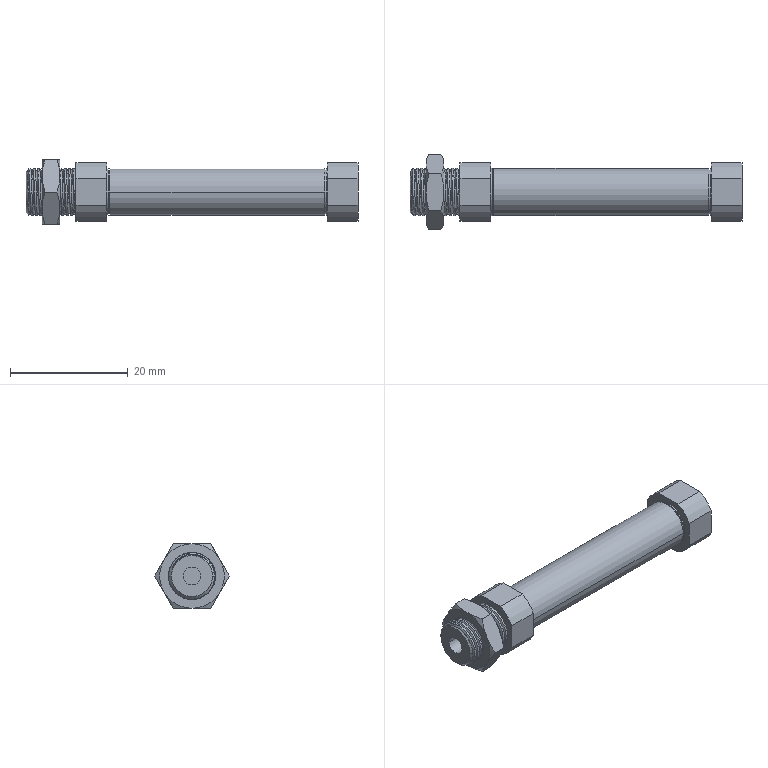Part | SolidWorks | 1 solid | 117 faces | box 56.5 x 12.702 x 11 mm | volume 2893 mm3 | cylinder 63 | plane 30 | cone 18 | spline 6 | commonest cylinder face diameters 8 x33 2.5 x14 11 x8 3 x2 4 x2 7.5 x2